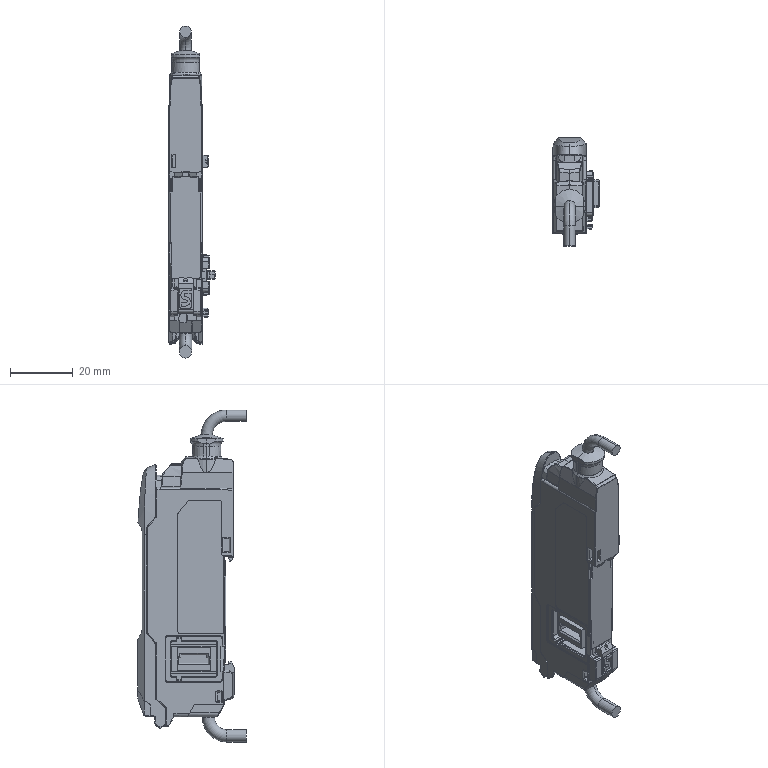Part | STEP file | [LR-XN12P]-Part-1 | 1 solid | 1272 faces | box 14.78 x 34.5 x 105.605 mm | volume 23972 mm3 | plane 728 | cylinder 323 | spline 166 | torus 20 | sphere 18 | cone 17 | commonest cylinder face diameters 0.4 x126 1 x44 0.6 x22 1.6 x15 2 x15 0.2 x13